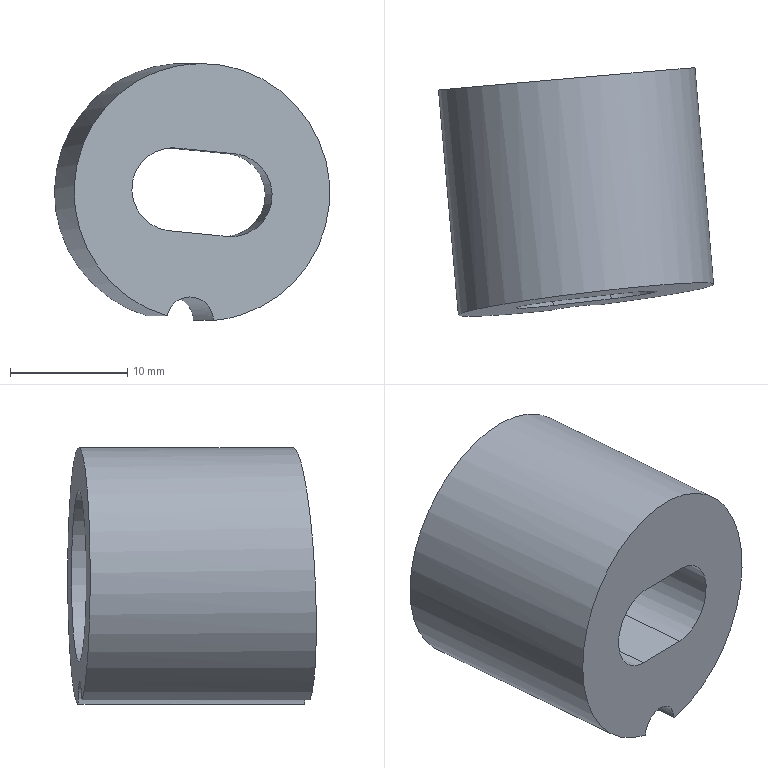Part | NX | features EKDE 22-20-12.10-7.100 2 | 1 solid | 10 faces | box 23.535 x 21.247 x 21.961 mm | volume 4548 mm3 | plane 5 | cylinder 5 | commonest cylinder face diameters 7.1 x2 4 x1 14.6 x1 22 x1
STEP:
#1=CARTESIAN_POINT('',(713.159,-54.83,-50.475));
#2=VERTEX_POINT('',#1);
#3=CARTESIAN_POINT('',(717.099,-54.375,-50.863));
#4=VERTEX_POINT('',#3);
#5=CARTESIAN_POINT('',(715.113,-54.614,-50.85));
#6=DIRECTION('',(-0.1195,0.9915,-0.05097));
#7=DIRECTION('',(0.5313,0.1073,0.8404));
#8=AXIS2_PLACEMENT_3D('',#5,#6,#7);
#9=ELLIPSE('',#8,2.004,2.);
#10=EDGE_CURVE('',#2,#4,#9,.T.);
#11=ORIENTED_EDGE('',*,*,#10,.T.);
#12=CARTESIAN_POINT('',(716.128,-53.928,-39.902));
#13=DIRECTION('',(-0.1195,0.9915,-0.05097));
#14=DIRECTION('',(0.5313,0.1073,0.8404));
#15=AXIS2_PLACEMENT_3D('',#12,#13,#14);
#16=ELLIPSE('',#15,11.02,11.);
#17=EDGE_CURVE('',#2,#4,#16,.T.);
#18=ORIENTED_EDGE('',*,*,#17,.F.);
#19=EDGE_LOOP('',(#11,#18));
#20=FACE_BOUND('',#19,.T.);
#21=CARTESIAN_POINT('',(713.328,-54.435,-43.192));
#22=VERTEX_POINT('',#21);
#23=CARTESIAN_POINT('',(718.273,-53.864,-43.679));
#24=VERTEX_POINT('',#23);
#25=CARTESIAN_POINT('',(715.22,-54.217,-43.378));
#26=DIRECTION('',(-0.9887,-0.1142,0.09735));
#27=VECTOR('',#26,1000.);
#28=LINE('',#25,#27);
#29=EDGE_CURVE('',#22,#24,#28,.F.);
#30=ORIENTED_EDGE('',*,*,#29,.F.);
#31=CARTESIAN_POINT('',(713.983,-53.993,-36.125));
#32=VERTEX_POINT('',#31);
#33=CARTESIAN_POINT('',(713.655,-54.214,-39.659));
#34=DIRECTION('',(-0.1195,0.9915,-0.05097));
#35=DIRECTION('',(0.5313,0.1073,0.8404));
#36=AXIS2_PLACEMENT_3D('',#33,#34,#35);
#37=ELLIPSE('',#36,3.557,3.55);
#38=EDGE_CURVE('',#22,#32,#37,.T.);
#39=ORIENTED_EDGE('',*,*,#38,.T.);
#40=CARTESIAN_POINT('',(718.928,-53.422,-36.612));
#41=VERTEX_POINT('',#40);
#42=CARTESIAN_POINT('',(715.865,-53.776,-36.311));
#43=DIRECTION('',(-0.9887,-0.1142,0.09735));
#44=VECTOR('',#43,1000.);
#45=LINE('',#42,#44);
#46=EDGE_CURVE('',#32,#41,#45,.F.);
#47=ORIENTED_EDGE('',*,*,#46,.T.);
#48=CARTESIAN_POINT('',(718.601,-53.643,-40.146));
#49=DIRECTION('',(-0.1195,0.9915,-0.05097));
#50=DIRECTION('',(0.5313,0.1073,0.8404));
#51=AXIS2_PLACEMENT_3D('',#48,#49,#50);
#52=ELLIPSE('',#51,3.557,3.55);
#53=EDGE_CURVE('',#41,#24,#52,.T.);
#54=ORIENTED_EDGE('',*,*,#53,.T.);
#55=EDGE_LOOP('',(#30,#39,#47,#54));
#56=FACE_BOUND('',#55,.T.);
#57=CARTESIAN_POINT('',(707.484,-59.507,-128.15));
#58=DIRECTION('',(-0.1195,0.9915,-0.05097));
#59=DIRECTION('',(0.06611,0.05918,0.9961));
#60=AXIS2_PLACEMENT_3D('',#57,#58,#59);
#61=PLANE('',#60);
#62=ADVANCED_FACE('',(#20,#56),#61,.F.);
#63=CARTESIAN_POINT('',(715.403,-34.991,-50.863));
#64=VERTEX_POINT('',#63);
#65=CARTESIAN_POINT('',(711.454,-35.336,-50.475));
#66=VERTEX_POINT('',#65);
#67=CARTESIAN_POINT('',(713.411,-35.165,-50.85));
#68=DIRECTION('',(0.08716,-0.9962,0.));
#69=DIRECTION('',(0.9962,0.08716,0.));
#70=AXIS2_PLACEMENT_3D('',#67,#68,#69);
#71=CIRCLE('',#70,2.);
#72=EDGE_CURVE('',#64,#66,#71,.T.);
#73=ORIENTED_EDGE('',*,*,#72,.T.);
#74=CARTESIAN_POINT('',(714.478,-35.072,-39.902));
#75=DIRECTION('',(0.08716,-0.9962,0.));
#76=DIRECTION('',(0.9962,0.08716,0.));
#77=AXIS2_PLACEMENT_3D('',#74,#75,#76);
#78=CIRCLE('',#77,11.);
#79=EDGE_CURVE('',#64,#66,#78,.T.);
#80=ORIENTED_EDGE('',*,*,#79,.F.);
#81=EDGE_LOOP('',(#73,#80));
#82=FACE_BOUND('',#81,.T.);
#83=CARTESIAN_POINT('',(707.206,-35.708,-39.902));
#84=VERTEX_POINT('',#83);
#85=CARTESIAN_POINT('',(714.478,-35.072,-39.902));
#86=DIRECTION('',(-0.08716,0.9962,0.));
#87=DIRECTION('',(-0.9962,-0.08716,0.));
#88=AXIS2_PLACEMENT_3D('',#85,#86,#87);
#89=CIRCLE('',#88,7.3);
#90=EDGE_CURVE('',#84,#84,#89,.T.);
#91=ORIENTED_EDGE('',*,*,#90,.F.);
#92=EDGE_LOOP('',(#91));
#93=FACE_BOUND('',#92,.T.);
#94=CARTESIAN_POINT('',(714.478,-35.072,-39.902));
#95=DIRECTION('',(-0.08716,0.9962,0.));
#96=DIRECTION('',(-0.9962,-0.08716,0.));
#97=AXIS2_PLACEMENT_3D('',#94,#95,#96);
#98=PLANE('',#97);
#99=ADVANCED_FACE('',(#82,#93),#98,.T.);
#100=CARTESIAN_POINT('',(712.326,-45.298,-50.475));
#101=DIRECTION('',(-0.08716,0.9962,0.));
#102=VECTOR('',#101,1000.);
#103=LINE('',#100,#102);
#104=EDGE_CURVE('',#2,#66,#103,.T.);
#105=ORIENTED_EDGE('',*,*,#104,.F.);
#106=ORIENTED_EDGE('',*,*,#17,.T.);
#107=CARTESIAN_POINT('',(716.275,-44.953,-50.863));
#108=DIRECTION('',(-0.08716,0.9962,0.));
#109=VECTOR('',#108,1000.);
#110=LINE('',#107,#109);
#111=EDGE_CURVE('',#64,#4,#110,.F.);
#112=ORIENTED_EDGE('',*,*,#111,.F.);
#113=ORIENTED_EDGE('',*,*,#79,.T.);
#114=EDGE_LOOP('',(#105,#106,#112,#113));
#115=FACE_BOUND('',#114,.T.);
#116=CARTESIAN_POINT('',(716.221,-54.996,-39.902));
#117=DIRECTION('',(-0.08716,0.9962,0.));
#118=DIRECTION('',(-0.9962,-0.08716,0.));
#119=AXIS2_PLACEMENT_3D('',#116,#117,#118);
#120=CYLINDRICAL_SURFACE('',#119,11.);
#121=ADVANCED_FACE('',(#115),#120,.T.);
#122=CARTESIAN_POINT('',(713.39,-47.213,-36.125));
#123=VERTEX_POINT('',#122);
#124=CARTESIAN_POINT('',(712.701,-47.273,-43.192));
#125=VERTEX_POINT('',#124);
#126=CARTESIAN_POINT('',(713.045,-47.243,-39.659));
#127=DIRECTION('',(0.08716,-0.9962,0.));
#128=DIRECTION('',(0.9962,0.08716,0.));
#129=AXIS2_PLACEMENT_3D('',#126,#127,#128);
#130=CIRCLE('',#129,3.55);
#131=EDGE_CURVE('',#123,#125,#130,.T.);
#132=ORIENTED_EDGE('',*,*,#131,.F.);
#133=CARTESIAN_POINT('',(714.741,-62.654,-36.125));
#134=DIRECTION('',(-0.08716,0.9962,0.));
#135=VECTOR('',#134,1000.);
#136=LINE('',#133,#135);
#137=EDGE_CURVE('',#32,#123,#136,.T.);
#138=ORIENTED_EDGE('',*,*,#137,.F.);
#139=ORIENTED_EDGE('',*,*,#38,.F.);
#140=CARTESIAN_POINT('',(714.052,-62.714,-43.192));
#141=DIRECTION('',(-0.08716,0.9962,0.));
#142=VECTOR('',#141,1000.);
#143=LINE('',#140,#142);
#144=EDGE_CURVE('',#22,#125,#143,.T.);
#145=ORIENTED_EDGE('',*,*,#144,.T.);
#146=EDGE_LOOP('',(#132,#138,#139,#145));
#147=FACE_BOUND('',#146,.T.);
#148=CARTESIAN_POINT('',(714.396,-62.684,-39.659));
#149=DIRECTION('',(-0.08716,0.9962,0.));
#150=DIRECTION('',(-0.9962,-0.08716,0.));
#151=AXIS2_PLACEMENT_3D('',#148,#149,#150);
#152=CYLINDRICAL_SURFACE('',#151,3.55);
#153=ADVANCED_FACE('',(#147),#152,.F.);
#154=CARTESIAN_POINT('',(717.658,-46.839,-43.679));
#155=VERTEX_POINT('',#154);
#156=CARTESIAN_POINT('',(719.009,-62.28,-43.679));
#157=DIRECTION('',(-0.08716,0.9962,0.));
#158=VECTOR('',#157,1000.);
#159=LINE('',#156,#158);
#160=EDGE_CURVE('',#24,#155,#159,.T.);
#161=ORIENTED_EDGE('',*,*,#160,.T.);
#162=CARTESIAN_POINT('',(717.658,-46.839,-43.679));
#163=DIRECTION('',(-0.9915,-0.08674,0.09739));
#164=VECTOR('',#163,1000.);
#165=LINE('',#162,#164);
#166=EDGE_CURVE('',#155,#125,#165,.T.);
#167=ORIENTED_EDGE('',*,*,#166,.T.);
#168=ORIENTED_EDGE('',*,*,#144,.F.);
#169=ORIENTED_EDGE('',*,*,#29,.T.);
#170=EDGE_LOOP('',(#161,#167,#168,#169));
#171=FACE_BOUND('',#170,.T.);
#172=CARTESIAN_POINT('',(719.009,-62.28,-43.679));
#173=DIRECTION('',(-0.09702,-0.008488,-0.9952));
#174=DIRECTION('',(-0.9953,0.,0.09702));
#175=AXIS2_PLACEMENT_3D('',#172,#173,#174);
#176=PLANE('',#175);
#177=ADVANCED_FACE('',(#171),#176,.F.);
#178=CARTESIAN_POINT('',(718.347,-46.779,-36.612));
#179=VERTEX_POINT('',#178);
#180=CARTESIAN_POINT('',(718.003,-46.809,-40.146));
#181=DIRECTION('',(0.08716,-0.9962,0.));
#182=DIRECTION('',(0.9962,0.08716,0.));
#183=AXIS2_PLACEMENT_3D('',#180,#181,#182);
#184=CIRCLE('',#183,3.55);
#185=EDGE_CURVE('',#155,#179,#184,.T.);
#186=ORIENTED_EDGE('',*,*,#185,.F.);
#187=ORIENTED_EDGE('',*,*,#160,.F.);
#188=ORIENTED_EDGE('',*,*,#53,.F.);
#189=CARTESIAN_POINT('',(719.698,-62.22,-36.612));
#190=DIRECTION('',(-0.08716,0.9962,0.));
#191=VECTOR('',#190,1000.);
#192=LINE('',#189,#191);
#193=EDGE_CURVE('',#41,#179,#192,.T.);
#194=ORIENTED_EDGE('',*,*,#193,.T.);
#195=EDGE_LOOP('',(#186,#187,#188,#194));
#196=FACE_BOUND('',#195,.T.);
#197=CARTESIAN_POINT('',(719.354,-62.25,-40.146));
#198=DIRECTION('',(-0.08716,0.9962,0.));
#199=DIRECTION('',(-0.9962,-0.08716,0.));
#200=AXIS2_PLACEMENT_3D('',#197,#198,#199);
#201=CYLINDRICAL_SURFACE('',#200,3.55);
#202=ADVANCED_FACE('',(#196),#201,.F.);
#203=CARTESIAN_POINT('',(718.347,-46.779,-36.612));
#204=DIRECTION('',(-0.9915,-0.08674,0.09739));
#205=VECTOR('',#204,1000.);
#206=LINE('',#203,#205);
#207=EDGE_CURVE('',#179,#123,#206,.T.);
#208=ORIENTED_EDGE('',*,*,#207,.F.);
#209=ORIENTED_EDGE('',*,*,#193,.F.);
#210=ORIENTED_EDGE('',*,*,#46,.F.);
#211=ORIENTED_EDGE('',*,*,#137,.T.);
#212=EDGE_LOOP('',(#208,#209,#210,#211));
#213=FACE_BOUND('',#212,.T.);
#214=CARTESIAN_POINT('',(719.698,-62.22,-36.612));
#215=DIRECTION('',(-0.09702,-0.008488,-0.9952));
#216=DIRECTION('',(-0.9953,0.,0.09702));
#217=AXIS2_PLACEMENT_3D('',#214,#215,#216);
#218=PLANE('',#217);
#219=ADVANCED_FACE('',(#213),#218,.T.);
#220=ORIENTED_EDGE('',*,*,#131,.T.);
#221=ORIENTED_EDGE('',*,*,#166,.F.);
#222=ORIENTED_EDGE('',*,*,#185,.T.);
#223=ORIENTED_EDGE('',*,*,#207,.T.);
#224=EDGE_LOOP('',(#220,#221,#222,#223));
#225=FACE_BOUND('',#224,.T.);
#226=CARTESIAN_POINT('',(708.252,-47.662,-39.902));
#227=VERTEX_POINT('',#226);
#228=CARTESIAN_POINT('',(715.524,-47.026,-39.902));
#229=DIRECTION('',(-0.08716,0.9962,0.));
#230=DIRECTION('',(-0.9962,-0.08716,0.));
#231=AXIS2_PLACEMENT_3D('',#228,#229,#230);
#232=CIRCLE('',#231,7.3);
#233=EDGE_CURVE('',#227,#227,#232,.T.);
#234=ORIENTED_EDGE('',*,*,#233,.T.);
#235=EDGE_LOOP('',(#234));
#236=FACE_BOUND('',#235,.T.);
#237=CARTESIAN_POINT('',(715.524,-47.026,-39.902));
#238=DIRECTION('',(0.08716,-0.9962,0.));
#239=DIRECTION('',(0.9962,0.08716,0.));
#240=AXIS2_PLACEMENT_3D('',#237,#238,#239);
#241=PLANE('',#240);
#242=ADVANCED_FACE('',(#225,#236),#241,.F.);
#243=ORIENTED_EDGE('',*,*,#90,.T.);
#244=EDGE_LOOP('',(#243));
#245=FACE_BOUND('',#244,.T.);
#246=ORIENTED_EDGE('',*,*,#233,.F.);
#247=EDGE_LOOP('',(#246));
#248=FACE_BOUND('',#247,.T.);
#249=CARTESIAN_POINT('',(715.524,-47.026,-39.902));
#250=DIRECTION('',(-0.08716,0.9962,0.));
#251=DIRECTION('',(-0.9962,-0.08716,0.));
#252=AXIS2_PLACEMENT_3D('',#249,#250,#251);
#253=CYLINDRICAL_SURFACE('',#252,7.3);
#254=ADVANCED_FACE('',(#245,#248),#253,.F.);
#255=ORIENTED_EDGE('',*,*,#104,.T.);
#256=ORIENTED_EDGE('',*,*,#72,.F.);
#257=ORIENTED_EDGE('',*,*,#111,.T.);
#258=ORIENTED_EDGE('',*,*,#10,.F.);
#259=EDGE_LOOP('',(#255,#256,#257,#258));
#260=FACE_BOUND('',#259,.T.);
#261=CARTESIAN_POINT('',(715.154,-55.089,-50.85));
#262=DIRECTION('',(-0.08716,0.9962,0.));
#263=DIRECTION('',(-0.9962,-0.08716,0.));
#264=AXIS2_PLACEMENT_3D('',#261,#262,#263);
#265=CYLINDRICAL_SURFACE('',#264,2.);
#266=ADVANCED_FACE('',(#260),#265,.F.);
#267=CLOSED_SHELL('',(#62,#99,#121,#153,#177,#202,#219,#242,#254,#266));
#268=MANIFOLD_SOLID_BREP('',#267);
#269=(LENGTH_UNIT()NAMED_UNIT(*)SI_UNIT(.MILLI.,.METRE.));
#270=UNCERTAINTY_MEASURE_WITH_UNIT(LENGTH_MEASURE(0.00001),#269,'','');
#271=(NAMED_UNIT(*)PLANE_ANGLE_UNIT()SI_UNIT($,.RADIAN.));
#272=(NAMED_UNIT(*)SI_UNIT($,.STERADIAN.)SOLID_ANGLE_UNIT());
#273=(GEOMETRIC_REPRESENTATION_CONTEXT(3)GLOBAL_UNCERTAINTY_ASSIGNED_CONTEXT((#270))GLOBAL_UNIT_ASSIGNED_CONTEXT((#269,#271,#272))REPRESENTATION_CONTEXT('',''));
#274=ADVANCED_BREP_SHAPE_REPRESENTATION('',(#268),#273);